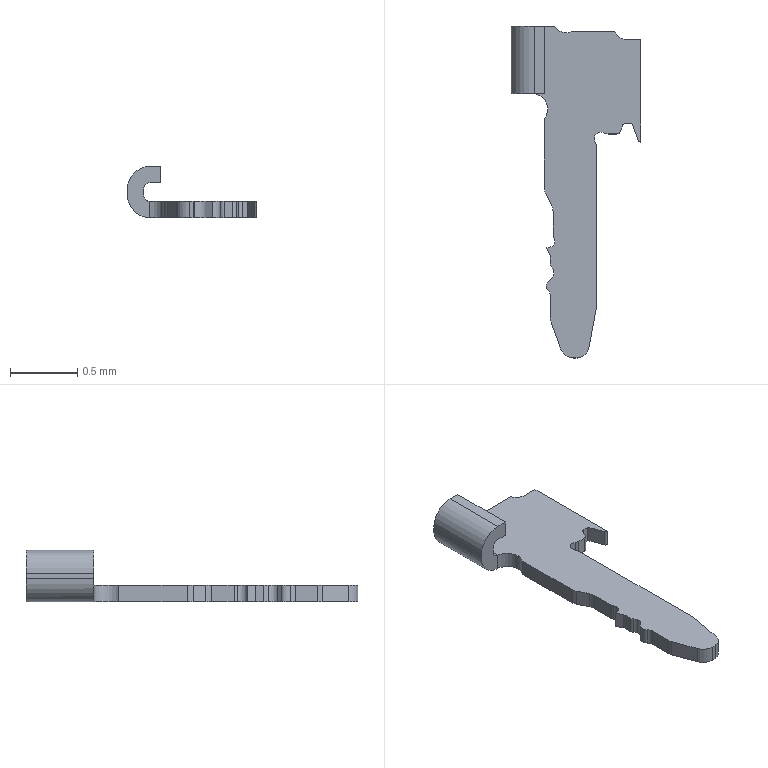Part | Creo | 1 solid | 53 faces | box 0.96 x 2.46 x 0.38 mm | volume 0.1619 mm3 | plane 29 | cylinder 24 | commonest cylinder face diameters 0.1 x11 0.2 x7 0.06 x2 0.34 x2 0.038 x1 0.232 x1